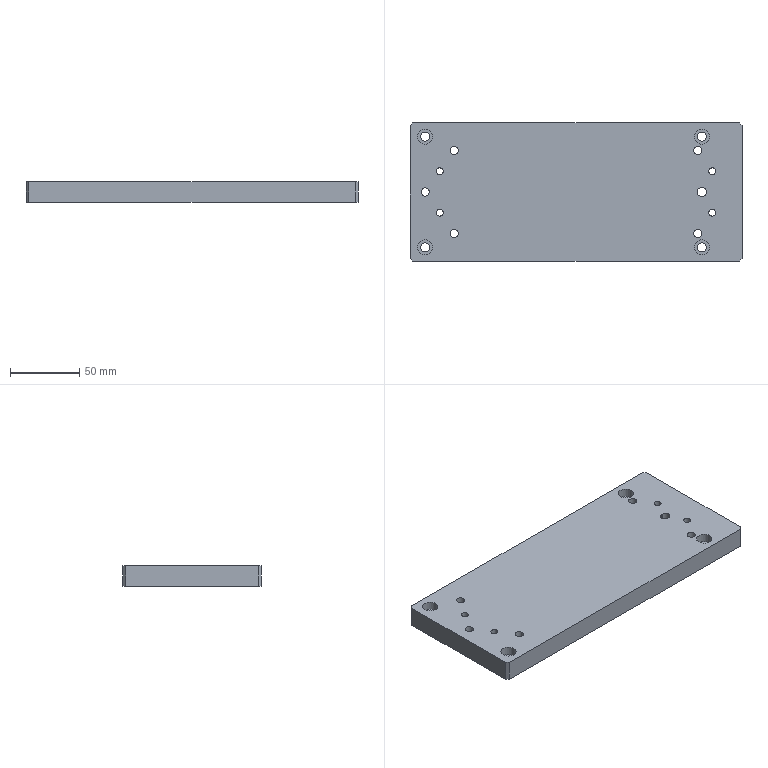CAM job | NX | 3-axis milling, drilling | part box 240 x 100 x 15 mm | stock box 245 x 100 x 20 mm
Tools:
number,name,description,diameter,corner_radius,flute_length,length,flutes
4,D4,平底铣刀-粗,4.0,0.0,25.0,75.0,2
6,D6,平底铣刀-粗,6.0,0.0,25.0,75.0,2
9,D10,平底铣刀-粗,10.0,0.0,35.0,75.0,2
11,D4-J,平底铣刀-精,4.0,0.0,50.0,75.0,2
7,D6-J,平底铣刀-精,6.0,0.0,25.0,75.0,2
10,D10-J,平底铣刀-精,10.0,0.0,35.0,75.0,2
1,D80R0.8_FACEMILL,圆鼻刀-粗,80.0,0.8,50.0,75.0,2
1,D80R0.8_FACEMILL-J,圆鼻刀-精,80.0,0.8,50.0,75.0,2
2,D6_CHAMFERTOOL,倒角刀,6.0,0.0,3.0,25.0,2
22,M6X1.0,丝锥,5.0,0.0,35.0,50.0,2
19,D6_REAMER,Drilling Tool,6.0,0.0,75.0,100.0,6
15,ZT5.1,钻头,5.1,0.0,35.0,50.0,2
18,ZT6.6,钻头,6.6,0.0,35.0,50.0,2
17,ZT5.9,Drilling Tool,5.9,0.0,35.0,50.0,2
Operations:
program,operation,operation_type,tool,method,geometry_group,spindle_rpm,surface_speed,feed_per_tooth,feed_cut,feed_plunge,cut_length_mm,path_length_mm,cut_time_min,machine_time_min
B,FLOORWALL_FACEMILL_ROUGH_COPY,VolumeBased25DMillingOperation,D80R0.8_FACEMILL-J,LAYERED_ROUGH-DEPTHK-STEPG,W-B,2800.0,703.696,0.5357,3000.0,100.0,3533.487,3806.711,1.178,1.205
B,FLOORWALL_FACEMILL_FINISH_COPY,VolumeBased25DMillingOperation,D80R0.8_FACEMILL-J,SIDEEDGE_FINISH-DEPTHK-STEPG,W-B,4000.0,1005.28,0.125,1000.0,100.0,706.11,802.11,0.7061,0.7157
B,MILL_CHAMFER_4,PlanarMilling,D6_CHAMFERTOOL,METHOD,W-B,8000.0,150.796,0.0375,600.0,100.0,75.821,740.029,0.1264,0.1928
B,PLANAR_DEBURR_6X45L_COPY,SurfaceContour,D6_CHAMFERTOOL,CLIMB_CHAMFER-DEPTH0-STEPG,W-B,6500.0,122.519,0.1154,1500.0,100.0,911.648,1763.9,0.6078,0.693
A,TOP_FACE,FaceMilling,D80R0.8_FACEMILL,SIDEEDGE_FINISH-DEPTHK-STEPG,W-A,4500.0,1385.0,0.1667,1500.0,100.0,1064.0,1160.0,0.7093,0.7189
A,CONTOUR_ROUGH_2,VolumeBased25DMillingOperation,D10,METHOD,W-A,8000.0,251.327,0.375,6000.0,80.0,14856.025,14969.525,2.476,2.487
A,SPOT-DEPTH0.8,Operation,D6_CHAMFERTOOL,NONE,W-A,8000.0,150.796,0.0312,500.0,90.0,23.4,554.456,0.0468,0.0999
A,SPOT-DEPTH0.8_COPY,Operation,D6_CHAMFERTOOL,NONE,W-A,8000.0,150.796,0.0312,500.0,90.0,1.8,103.6,0.0036,0.0138
A,THRUHOLE-M6_TAPPILOT,Operation,ZT5.1,NONE,W-A,2800.0,43.982,0.0625,350.0,90.0,96.0,552.036,0.2743,0.3199
A,THRUHOLE-FINISH6.0_PREDRILL,Operation,ZT5.9,NONE,W-A,2500.0,46.339,0.05,250.0,90.0,103.516,620.31,0.4141,0.4657
A,THRUHOLE-FINISH6.0_PREDRILL_COPY,Operation,ZT5.9,NONE,W-A,2500.0,46.339,0.05,250.0,90.0,20.703,141.406,0.0828,0.0949
A,COUNTERSINK-DRILL_SEG0,Operation,ZT6.6,NONE,W-A,1200.0,24.881,0.1042,250.0,90.0,79.931,622.878,0.3197,0.374
A,THRUSLOT_ROUGH_1,VolumeBased25DMillingOperation,D4,METHOD,W-A,12000.0,150.796,0.0208,500.0,100.0,830.423,943.823,1.661,1.672
A,HOLE_ROUGH_D6_1,CylinderMilling,D6,NONE,W-A,8000.0,150.796,0.075,1200.0,100.0,923.332,1706.932,0.7694,0.8478
A,HOLE_FINISH_D6_1,CylinderMilling,D6-J,FINISH_STEPDEPTH_OFF,W-A,8000.0,150.796,0.0312,500.0,100.0,178.461,964.061,0.3569,0.4355
A,SELECTBODYONLY,SurfaceContour,D6_CHAMFERTOOL,METHOD,W-A,8000.0,150.796,0.1875,3000.0,100.0,714.443,1010.488,0.2381,0.2678
A,MILL_CHAMFER_1,PlanarMilling,D6_CHAMFERTOOL,METHOD,W-A,8000.0,150.796,0.0312,500.0,100.0,79.753,741.563,0.1595,0.2257
A,MILL_CHAMFER_2,PlanarMilling,D6_CHAMFERTOOL,METHOD,W-A,8000.0,150.796,0.0312,500.0,100.0,104.819,920.582,0.2096,0.2912
A,MILL_CHAMFER_3,PlanarMilling,D6_CHAMFERTOOL,NONE,W-A,8000.0,150.796,0.05,800.0,100.0,173.57,924.987,0.217,0.2921
A,REAM_HOLE,Operation,D6_REAMER,METHOD,W-A,500.0,9.425,0.0167,50.0,0.0,85.0,583.278,1.7,1.75
A,THRUHOLE-TAPM6,Operation,M6X1.0,METHOD,W-A,500.0,7.854,0.001,1.0,90.0,78.0,516.036,78.0,78.044
A,SLOT_FINISH_1,VolumeBased25DMillingOperation,D4-J,METHOD,W-A,8000.0,100.531,0.0125,200.0,100.0,31.798,182.266,0.159,0.174
A,CONTOUR_SEMIFINISH_2,VolumeBased25DMillingOperation,D10-J,METHOD,W-A,9000.0,169.646,0.0667,1200.0,100.0,1423.376,1668.89,1.186,1.211
A,FLOORWALL_FINISH_SIDE-MID_COPY,VolumeBased25DMillingOperation,D10-J,SIDEEDGE_FINISH-DEPTHK-STEPG,W-A,8000.0,251.32,0.0625,1000.0,100.0,1016.45,1709.025,1.016,1.086